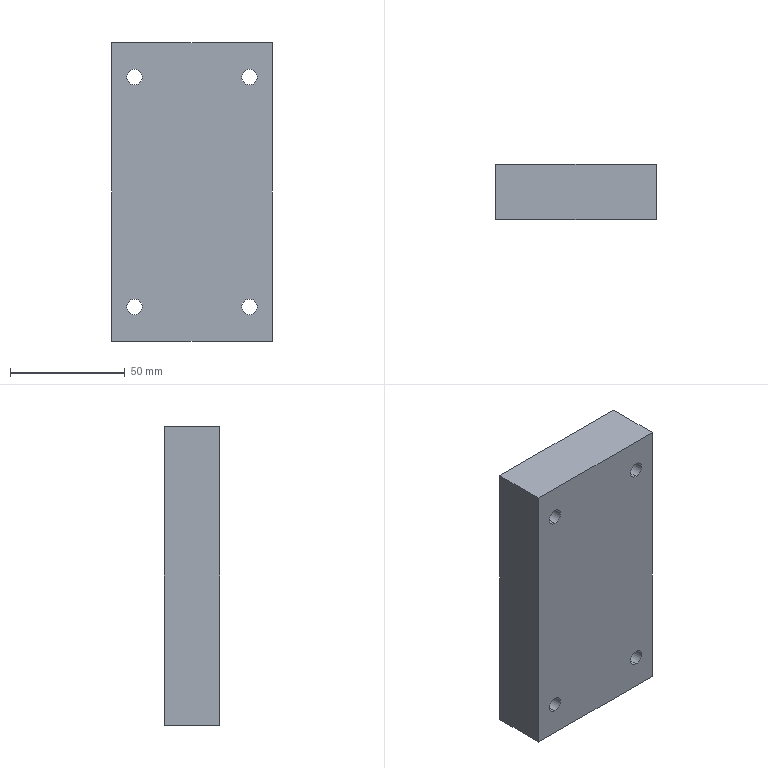Part | SolidWorks | features Extrusion 1, HoleWzd 1 | 1 solid | 14 faces | box 70 x 24 x 130 mm | volume 214914 mm3 | cylinder 8 | plane 6 | commonest cylinder face diameters 6.8 x8
STEP:
#1=CARTESIAN_POINT('',(-25.,0.,46.6));
#2=VERTEX_POINT('',#1);
#3=CARTESIAN_POINT('',(-25.,0.,53.4));
#4=VERTEX_POINT('',#3);
#5=CARTESIAN_POINT('',(-25.,0.,50.));
#6=DIRECTION('',(0.,1.,0.));
#7=DIRECTION('',(0.,0.,1.));
#8=AXIS2_PLACEMENT_3D('',#5,#6,#7);
#9=CIRCLE('',#8,3.4);
#10=EDGE_CURVE('',#2,#4,#9,.T.);
#11=ORIENTED_EDGE('',*,*,#10,.F.);
#12=CARTESIAN_POINT('',(-25.,24.,46.6));
#13=VERTEX_POINT('',#12);
#14=CARTESIAN_POINT('',(-25.,24.,46.6));
#15=DIRECTION('',(0.,1.,0.));
#16=VECTOR('',#15,1000.);
#17=LINE('',#14,#16);
#18=EDGE_CURVE('',#2,#13,#17,.T.);
#19=ORIENTED_EDGE('',*,*,#18,.T.);
#20=CARTESIAN_POINT('',(-25.,24.,53.4));
#21=VERTEX_POINT('',#20);
#22=CARTESIAN_POINT('',(-25.,24.,50.));
#23=DIRECTION('',(0.,1.,0.));
#24=DIRECTION('',(0.,0.,1.));
#25=AXIS2_PLACEMENT_3D('',#22,#23,#24);
#26=CIRCLE('',#25,3.4);
#27=EDGE_CURVE('',#13,#21,#26,.T.);
#28=ORIENTED_EDGE('',*,*,#27,.T.);
#29=CARTESIAN_POINT('',(-25.,24.,53.4));
#30=DIRECTION('',(0.,1.,0.));
#31=VECTOR('',#30,1000.);
#32=LINE('',#29,#31);
#33=EDGE_CURVE('',#4,#21,#32,.T.);
#34=ORIENTED_EDGE('',*,*,#33,.F.);
#35=EDGE_LOOP('',(#11,#19,#28,#34));
#36=FACE_OUTER_BOUND('',#35,.T.);
#37=CARTESIAN_POINT('',(-25.,24.,50.));
#38=DIRECTION('',(0.,1.,0.));
#39=DIRECTION('',(0.,0.,1.));
#40=AXIS2_PLACEMENT_3D('',#37,#38,#39);
#41=CYLINDRICAL_SURFACE('',#40,3.4);
#42=ADVANCED_FACE('',(#36),#41,.F.);
#43=CARTESIAN_POINT('',(-25.,0.,-53.4));
#44=VERTEX_POINT('',#43);
#45=CARTESIAN_POINT('',(-25.,0.,-46.6));
#46=VERTEX_POINT('',#45);
#47=CARTESIAN_POINT('',(-25.,0.,-50.));
#48=DIRECTION('',(0.,1.,0.));
#49=DIRECTION('',(0.,0.,1.));
#50=AXIS2_PLACEMENT_3D('',#47,#48,#49);
#51=CIRCLE('',#50,3.4);
#52=EDGE_CURVE('',#44,#46,#51,.T.);
#53=ORIENTED_EDGE('',*,*,#52,.F.);
#54=CARTESIAN_POINT('',(-25.,24.,-53.4));
#55=VERTEX_POINT('',#54);
#56=CARTESIAN_POINT('',(-25.,24.,-53.4));
#57=DIRECTION('',(0.,1.,0.));
#58=VECTOR('',#57,1000.);
#59=LINE('',#56,#58);
#60=EDGE_CURVE('',#44,#55,#59,.T.);
#61=ORIENTED_EDGE('',*,*,#60,.T.);
#62=CARTESIAN_POINT('',(-25.,24.,-46.6));
#63=VERTEX_POINT('',#62);
#64=CARTESIAN_POINT('',(-25.,24.,-50.));
#65=DIRECTION('',(0.,1.,0.));
#66=DIRECTION('',(0.,0.,1.));
#67=AXIS2_PLACEMENT_3D('',#64,#65,#66);
#68=CIRCLE('',#67,3.4);
#69=EDGE_CURVE('',#55,#63,#68,.T.);
#70=ORIENTED_EDGE('',*,*,#69,.T.);
#71=CARTESIAN_POINT('',(-25.,24.,-46.6));
#72=DIRECTION('',(0.,1.,0.));
#73=VECTOR('',#72,1000.);
#74=LINE('',#71,#73);
#75=EDGE_CURVE('',#46,#63,#74,.T.);
#76=ORIENTED_EDGE('',*,*,#75,.F.);
#77=EDGE_LOOP('',(#53,#61,#70,#76));
#78=FACE_OUTER_BOUND('',#77,.T.);
#79=CARTESIAN_POINT('',(-25.,24.,-50.));
#80=DIRECTION('',(0.,1.,0.));
#81=DIRECTION('',(0.,0.,1.));
#82=AXIS2_PLACEMENT_3D('',#79,#80,#81);
#83=CYLINDRICAL_SURFACE('',#82,3.4);
#84=ADVANCED_FACE('',(#78),#83,.F.);
#85=CARTESIAN_POINT('',(25.,0.,-53.4));
#86=VERTEX_POINT('',#85);
#87=CARTESIAN_POINT('',(25.,0.,-46.6));
#88=VERTEX_POINT('',#87);
#89=CARTESIAN_POINT('',(25.,0.,-50.));
#90=DIRECTION('',(0.,1.,0.));
#91=DIRECTION('',(0.,0.,1.));
#92=AXIS2_PLACEMENT_3D('',#89,#90,#91);
#93=CIRCLE('',#92,3.4);
#94=EDGE_CURVE('',#86,#88,#93,.T.);
#95=ORIENTED_EDGE('',*,*,#94,.F.);
#96=CARTESIAN_POINT('',(25.,24.,-53.4));
#97=VERTEX_POINT('',#96);
#98=CARTESIAN_POINT('',(25.,24.,-53.4));
#99=DIRECTION('',(0.,1.,0.));
#100=VECTOR('',#99,1000.);
#101=LINE('',#98,#100);
#102=EDGE_CURVE('',#86,#97,#101,.T.);
#103=ORIENTED_EDGE('',*,*,#102,.T.);
#104=CARTESIAN_POINT('',(25.,24.,-46.6));
#105=VERTEX_POINT('',#104);
#106=CARTESIAN_POINT('',(25.,24.,-50.));
#107=DIRECTION('',(0.,1.,0.));
#108=DIRECTION('',(0.,0.,1.));
#109=AXIS2_PLACEMENT_3D('',#106,#107,#108);
#110=CIRCLE('',#109,3.4);
#111=EDGE_CURVE('',#97,#105,#110,.T.);
#112=ORIENTED_EDGE('',*,*,#111,.T.);
#113=CARTESIAN_POINT('',(25.,24.,-46.6));
#114=DIRECTION('',(0.,1.,0.));
#115=VECTOR('',#114,1000.);
#116=LINE('',#113,#115);
#117=EDGE_CURVE('',#88,#105,#116,.T.);
#118=ORIENTED_EDGE('',*,*,#117,.F.);
#119=EDGE_LOOP('',(#95,#103,#112,#118));
#120=FACE_OUTER_BOUND('',#119,.T.);
#121=CARTESIAN_POINT('',(25.,24.,-50.));
#122=DIRECTION('',(0.,1.,0.));
#123=DIRECTION('',(0.,0.,1.));
#124=AXIS2_PLACEMENT_3D('',#121,#122,#123);
#125=CYLINDRICAL_SURFACE('',#124,3.4);
#126=ADVANCED_FACE('',(#120),#125,.F.);
#127=CARTESIAN_POINT('',(25.,0.,46.6));
#128=VERTEX_POINT('',#127);
#129=CARTESIAN_POINT('',(25.,0.,53.4));
#130=VERTEX_POINT('',#129);
#131=CARTESIAN_POINT('',(25.,0.,50.));
#132=DIRECTION('',(0.,1.,0.));
#133=DIRECTION('',(0.,0.,1.));
#134=AXIS2_PLACEMENT_3D('',#131,#132,#133);
#135=CIRCLE('',#134,3.4);
#136=EDGE_CURVE('',#128,#130,#135,.T.);
#137=ORIENTED_EDGE('',*,*,#136,.F.);
#138=CARTESIAN_POINT('',(25.,24.,46.6));
#139=VERTEX_POINT('',#138);
#140=CARTESIAN_POINT('',(25.,24.,46.6));
#141=DIRECTION('',(0.,1.,0.));
#142=VECTOR('',#141,1000.);
#143=LINE('',#140,#142);
#144=EDGE_CURVE('',#128,#139,#143,.T.);
#145=ORIENTED_EDGE('',*,*,#144,.T.);
#146=CARTESIAN_POINT('',(25.,24.,53.4));
#147=VERTEX_POINT('',#146);
#148=CARTESIAN_POINT('',(25.,24.,50.));
#149=DIRECTION('',(0.,1.,0.));
#150=DIRECTION('',(0.,0.,1.));
#151=AXIS2_PLACEMENT_3D('',#148,#149,#150);
#152=CIRCLE('',#151,3.4);
#153=EDGE_CURVE('',#139,#147,#152,.T.);
#154=ORIENTED_EDGE('',*,*,#153,.T.);
#155=CARTESIAN_POINT('',(25.,24.,53.4));
#156=DIRECTION('',(0.,1.,0.));
#157=VECTOR('',#156,1000.);
#158=LINE('',#155,#157);
#159=EDGE_CURVE('',#130,#147,#158,.T.);
#160=ORIENTED_EDGE('',*,*,#159,.F.);
#161=EDGE_LOOP('',(#137,#145,#154,#160));
#162=FACE_OUTER_BOUND('',#161,.T.);
#163=CARTESIAN_POINT('',(25.,24.,50.));
#164=DIRECTION('',(0.,1.,0.));
#165=DIRECTION('',(0.,0.,1.));
#166=AXIS2_PLACEMENT_3D('',#163,#164,#165);
#167=CYLINDRICAL_SURFACE('',#166,3.4);
#168=ADVANCED_FACE('',(#162),#167,.F.);
#169=CARTESIAN_POINT('',(35.,0.,65.));
#170=VERTEX_POINT('',#169);
#171=CARTESIAN_POINT('',(35.,0.,-65.));
#172=VERTEX_POINT('',#171);
#173=CARTESIAN_POINT('',(35.,0.,65.));
#174=DIRECTION('',(0.,0.,-1.));
#175=VECTOR('',#174,1000.);
#176=LINE('',#173,#175);
#177=EDGE_CURVE('',#170,#172,#176,.T.);
#178=ORIENTED_EDGE('',*,*,#177,.T.);
#179=CARTESIAN_POINT('',(35.,24.,-65.));
#180=VERTEX_POINT('',#179);
#181=CARTESIAN_POINT('',(35.,24.,-65.));
#182=DIRECTION('',(0.,-1.,0.));
#183=VECTOR('',#182,1000.);
#184=LINE('',#181,#183);
#185=EDGE_CURVE('',#180,#172,#184,.T.);
#186=ORIENTED_EDGE('',*,*,#185,.F.);
#187=CARTESIAN_POINT('',(35.,24.,65.));
#188=VERTEX_POINT('',#187);
#189=CARTESIAN_POINT('',(35.,24.,65.));
#190=DIRECTION('',(0.,0.,-1.));
#191=VECTOR('',#190,1000.);
#192=LINE('',#189,#191);
#193=EDGE_CURVE('',#188,#180,#192,.T.);
#194=ORIENTED_EDGE('',*,*,#193,.F.);
#195=CARTESIAN_POINT('',(35.,24.,65.));
#196=DIRECTION('',(0.,-1.,0.));
#197=VECTOR('',#196,1000.);
#198=LINE('',#195,#197);
#199=EDGE_CURVE('',#188,#170,#198,.T.);
#200=ORIENTED_EDGE('',*,*,#199,.T.);
#201=EDGE_LOOP('',(#178,#186,#194,#200));
#202=FACE_OUTER_BOUND('',#201,.T.);
#203=CARTESIAN_POINT('',(35.,24.,65.));
#204=DIRECTION('',(-1.,0.,0.));
#205=DIRECTION('',(0.,0.,1.));
#206=AXIS2_PLACEMENT_3D('',#203,#204,#205);
#207=PLANE('',#206);
#208=ADVANCED_FACE('',(#202),#207,.F.);
#209=CARTESIAN_POINT('',(-35.,0.,-65.));
#210=VERTEX_POINT('',#209);
#211=CARTESIAN_POINT('',(-35.,0.,-65.));
#212=DIRECTION('',(-1.,0.,0.));
#213=VECTOR('',#212,1000.);
#214=LINE('',#211,#213);
#215=EDGE_CURVE('',#172,#210,#214,.T.);
#216=ORIENTED_EDGE('',*,*,#215,.T.);
#217=CARTESIAN_POINT('',(-35.,24.,-65.));
#218=VERTEX_POINT('',#217);
#219=CARTESIAN_POINT('',(-35.,24.,-65.));
#220=DIRECTION('',(0.,-1.,0.));
#221=VECTOR('',#220,1000.);
#222=LINE('',#219,#221);
#223=EDGE_CURVE('',#218,#210,#222,.T.);
#224=ORIENTED_EDGE('',*,*,#223,.F.);
#225=CARTESIAN_POINT('',(-35.,24.,-65.));
#226=DIRECTION('',(-1.,0.,0.));
#227=VECTOR('',#226,1000.);
#228=LINE('',#225,#227);
#229=EDGE_CURVE('',#180,#218,#228,.T.);
#230=ORIENTED_EDGE('',*,*,#229,.F.);
#231=ORIENTED_EDGE('',*,*,#185,.T.);
#232=EDGE_LOOP('',(#216,#224,#230,#231));
#233=FACE_OUTER_BOUND('',#232,.T.);
#234=CARTESIAN_POINT('',(-35.,24.,-65.));
#235=DIRECTION('',(0.,0.,1.));
#236=DIRECTION('',(1.,0.,0.));
#237=AXIS2_PLACEMENT_3D('',#234,#235,#236);
#238=PLANE('',#237);
#239=ADVANCED_FACE('',(#233),#238,.F.);
#240=CARTESIAN_POINT('',(-35.,0.,65.));
#241=VERTEX_POINT('',#240);
#242=CARTESIAN_POINT('',(-35.,0.,65.));
#243=DIRECTION('',(0.,0.,1.));
#244=VECTOR('',#243,1000.);
#245=LINE('',#242,#244);
#246=EDGE_CURVE('',#210,#241,#245,.T.);
#247=ORIENTED_EDGE('',*,*,#246,.T.);
#248=CARTESIAN_POINT('',(-35.,24.,65.));
#249=VERTEX_POINT('',#248);
#250=CARTESIAN_POINT('',(-35.,24.,65.));
#251=DIRECTION('',(0.,-1.,0.));
#252=VECTOR('',#251,1000.);
#253=LINE('',#250,#252);
#254=EDGE_CURVE('',#249,#241,#253,.T.);
#255=ORIENTED_EDGE('',*,*,#254,.F.);
#256=CARTESIAN_POINT('',(-35.,24.,65.));
#257=DIRECTION('',(0.,0.,1.));
#258=VECTOR('',#257,1000.);
#259=LINE('',#256,#258);
#260=EDGE_CURVE('',#218,#249,#259,.T.);
#261=ORIENTED_EDGE('',*,*,#260,.F.);
#262=ORIENTED_EDGE('',*,*,#223,.T.);
#263=EDGE_LOOP('',(#247,#255,#261,#262));
#264=FACE_OUTER_BOUND('',#263,.T.);
#265=CARTESIAN_POINT('',(-35.,24.,65.));
#266=DIRECTION('',(1.,0.,0.));
#267=DIRECTION('',(0.,0.,-1.));
#268=AXIS2_PLACEMENT_3D('',#265,#266,#267);
#269=PLANE('',#268);
#270=ADVANCED_FACE('',(#264),#269,.F.);
#271=CARTESIAN_POINT('',(-35.,0.,65.));
#272=DIRECTION('',(1.,0.,0.));
#273=VECTOR('',#272,1000.);
#274=LINE('',#271,#273);
#275=EDGE_CURVE('',#241,#170,#274,.T.);
#276=ORIENTED_EDGE('',*,*,#275,.T.);
#277=ORIENTED_EDGE('',*,*,#199,.F.);
#278=CARTESIAN_POINT('',(-35.,24.,65.));
#279=DIRECTION('',(1.,0.,0.));
#280=VECTOR('',#279,1000.);
#281=LINE('',#278,#280);
#282=EDGE_CURVE('',#249,#188,#281,.T.);
#283=ORIENTED_EDGE('',*,*,#282,.F.);
#284=ORIENTED_EDGE('',*,*,#254,.T.);
#285=EDGE_LOOP('',(#276,#277,#283,#284));
#286=FACE_OUTER_BOUND('',#285,.T.);
#287=CARTESIAN_POINT('',(-35.,24.,65.));
#288=DIRECTION('',(0.,0.,-1.));
#289=DIRECTION('',(-1.,0.,0.));
#290=AXIS2_PLACEMENT_3D('',#287,#288,#289);
#291=PLANE('',#290);
#292=ADVANCED_FACE('',(#286),#291,.F.);
#293=CARTESIAN_POINT('',(-25.,24.,50.));
#294=DIRECTION('',(0.,1.,0.));
#295=DIRECTION('',(0.,0.,1.));
#296=AXIS2_PLACEMENT_3D('',#293,#294,#295);
#297=CIRCLE('',#296,3.4);
#298=EDGE_CURVE('',#21,#13,#297,.T.);
#299=ORIENTED_EDGE('',*,*,#298,.F.);
#300=ORIENTED_EDGE('',*,*,#27,.F.);
#301=EDGE_LOOP('',(#299,#300));
#302=FACE_BOUND('',#301,.T.);
#303=CARTESIAN_POINT('',(-25.,24.,-50.));
#304=DIRECTION('',(0.,1.,0.));
#305=DIRECTION('',(0.,0.,1.));
#306=AXIS2_PLACEMENT_3D('',#303,#304,#305);
#307=CIRCLE('',#306,3.4);
#308=EDGE_CURVE('',#63,#55,#307,.T.);
#309=ORIENTED_EDGE('',*,*,#308,.F.);
#310=ORIENTED_EDGE('',*,*,#69,.F.);
#311=EDGE_LOOP('',(#309,#310));
#312=FACE_BOUND('',#311,.T.);
#313=CARTESIAN_POINT('',(25.,24.,-50.));
#314=DIRECTION('',(0.,1.,0.));
#315=DIRECTION('',(0.,0.,1.));
#316=AXIS2_PLACEMENT_3D('',#313,#314,#315);
#317=CIRCLE('',#316,3.4);
#318=EDGE_CURVE('',#105,#97,#317,.T.);
#319=ORIENTED_EDGE('',*,*,#318,.F.);
#320=ORIENTED_EDGE('',*,*,#111,.F.);
#321=EDGE_LOOP('',(#319,#320));
#322=FACE_BOUND('',#321,.T.);
#323=CARTESIAN_POINT('',(25.,24.,50.));
#324=DIRECTION('',(0.,1.,0.));
#325=DIRECTION('',(0.,0.,1.));
#326=AXIS2_PLACEMENT_3D('',#323,#324,#325);
#327=CIRCLE('',#326,3.4);
#328=EDGE_CURVE('',#147,#139,#327,.T.);
#329=ORIENTED_EDGE('',*,*,#328,.F.);
#330=ORIENTED_EDGE('',*,*,#153,.F.);
#331=EDGE_LOOP('',(#329,#330));
#332=FACE_BOUND('',#331,.T.);
#333=ORIENTED_EDGE('',*,*,#193,.T.);
#334=ORIENTED_EDGE('',*,*,#229,.T.);
#335=ORIENTED_EDGE('',*,*,#260,.T.);
#336=ORIENTED_EDGE('',*,*,#282,.T.);
#337=EDGE_LOOP('',(#333,#334,#335,#336));
#338=FACE_OUTER_BOUND('',#337,.T.);
#339=CARTESIAN_POINT('',(0.,24.,0.));
#340=DIRECTION('',(0.,-1.,0.));
#341=DIRECTION('',(0.,0.,-1.));
#342=AXIS2_PLACEMENT_3D('',#339,#340,#341);
#343=PLANE('',#342);
#344=ADVANCED_FACE('',(#302,#312,#322,#332,#338),#343,.F.);
#345=CARTESIAN_POINT('',(-25.,0.,50.));
#346=DIRECTION('',(0.,1.,0.));
#347=DIRECTION('',(0.,0.,1.));
#348=AXIS2_PLACEMENT_3D('',#345,#346,#347);
#349=CIRCLE('',#348,3.4);
#350=EDGE_CURVE('',#4,#2,#349,.T.);
#351=ORIENTED_EDGE('',*,*,#350,.T.);
#352=ORIENTED_EDGE('',*,*,#10,.T.);
#353=EDGE_LOOP('',(#351,#352));
#354=FACE_BOUND('',#353,.T.);
#355=CARTESIAN_POINT('',(-25.,0.,-50.));
#356=DIRECTION('',(0.,1.,0.));
#357=DIRECTION('',(0.,0.,1.));
#358=AXIS2_PLACEMENT_3D('',#355,#356,#357);
#359=CIRCLE('',#358,3.4);
#360=EDGE_CURVE('',#46,#44,#359,.T.);
#361=ORIENTED_EDGE('',*,*,#360,.T.);
#362=ORIENTED_EDGE('',*,*,#52,.T.);
#363=EDGE_LOOP('',(#361,#362));
#364=FACE_BOUND('',#363,.T.);
#365=CARTESIAN_POINT('',(25.,0.,-50.));
#366=DIRECTION('',(0.,1.,0.));
#367=DIRECTION('',(0.,0.,1.));
#368=AXIS2_PLACEMENT_3D('',#365,#366,#367);
#369=CIRCLE('',#368,3.4);
#370=EDGE_CURVE('',#88,#86,#369,.T.);
#371=ORIENTED_EDGE('',*,*,#370,.T.);
#372=ORIENTED_EDGE('',*,*,#94,.T.);
#373=EDGE_LOOP('',(#371,#372));
#374=FACE_BOUND('',#373,.T.);
#375=CARTESIAN_POINT('',(25.,0.,50.));
#376=DIRECTION('',(0.,1.,0.));
#377=DIRECTION('',(0.,0.,1.));
#378=AXIS2_PLACEMENT_3D('',#375,#376,#377);
#379=CIRCLE('',#378,3.4);
#380=EDGE_CURVE('',#130,#128,#379,.T.);
#381=ORIENTED_EDGE('',*,*,#380,.T.);
#382=ORIENTED_EDGE('',*,*,#136,.T.);
#383=EDGE_LOOP('',(#381,#382));
#384=FACE_BOUND('',#383,.T.);
#385=ORIENTED_EDGE('',*,*,#177,.F.);
#386=ORIENTED_EDGE('',*,*,#275,.F.);
#387=ORIENTED_EDGE('',*,*,#246,.F.);
#388=ORIENTED_EDGE('',*,*,#215,.F.);
#389=EDGE_LOOP('',(#385,#386,#387,#388));
#390=FACE_OUTER_BOUND('',#389,.T.);
#391=CARTESIAN_POINT('',(0.,0.,0.));
#392=DIRECTION('',(0.,-1.,0.));
#393=DIRECTION('',(0.,0.,-1.));
#394=AXIS2_PLACEMENT_3D('',#391,#392,#393);
#395=PLANE('',#394);
#396=ADVANCED_FACE('',(#354,#364,#374,#384,#390),#395,.T.);
#397=ORIENTED_EDGE('',*,*,#144,.F.);
#398=ORIENTED_EDGE('',*,*,#380,.F.);
#399=ORIENTED_EDGE('',*,*,#159,.T.);
#400=ORIENTED_EDGE('',*,*,#328,.T.);
#401=EDGE_LOOP('',(#397,#398,#399,#400));
#402=FACE_OUTER_BOUND('',#401,.T.);
#403=CARTESIAN_POINT('',(25.,24.,50.));
#404=DIRECTION('',(0.,1.,0.));
#405=DIRECTION('',(0.,0.,1.));
#406=AXIS2_PLACEMENT_3D('',#403,#404,#405);
#407=CYLINDRICAL_SURFACE('',#406,3.4);
#408=ADVANCED_FACE('',(#402),#407,.F.);
#409=ORIENTED_EDGE('',*,*,#102,.F.);
#410=ORIENTED_EDGE('',*,*,#370,.F.);
#411=ORIENTED_EDGE('',*,*,#117,.T.);
#412=ORIENTED_EDGE('',*,*,#318,.T.);
#413=EDGE_LOOP('',(#409,#410,#411,#412));
#414=FACE_OUTER_BOUND('',#413,.T.);
#415=CARTESIAN_POINT('',(25.,24.,-50.));
#416=DIRECTION('',(0.,1.,0.));
#417=DIRECTION('',(0.,0.,1.));
#418=AXIS2_PLACEMENT_3D('',#415,#416,#417);
#419=CYLINDRICAL_SURFACE('',#418,3.4);
#420=ADVANCED_FACE('',(#414),#419,.F.);
#421=ORIENTED_EDGE('',*,*,#60,.F.);
#422=ORIENTED_EDGE('',*,*,#360,.F.);
#423=ORIENTED_EDGE('',*,*,#75,.T.);
#424=ORIENTED_EDGE('',*,*,#308,.T.);
#425=EDGE_LOOP('',(#421,#422,#423,#424));
#426=FACE_OUTER_BOUND('',#425,.T.);
#427=CARTESIAN_POINT('',(-25.,24.,-50.));
#428=DIRECTION('',(0.,1.,0.));
#429=DIRECTION('',(0.,0.,1.));
#430=AXIS2_PLACEMENT_3D('',#427,#428,#429);
#431=CYLINDRICAL_SURFACE('',#430,3.4);
#432=ADVANCED_FACE('',(#426),#431,.F.);
#433=ORIENTED_EDGE('',*,*,#18,.F.);
#434=ORIENTED_EDGE('',*,*,#350,.F.);
#435=ORIENTED_EDGE('',*,*,#33,.T.);
#436=ORIENTED_EDGE('',*,*,#298,.T.);
#437=EDGE_LOOP('',(#433,#434,#435,#436));
#438=FACE_OUTER_BOUND('',#437,.T.);
#439=CARTESIAN_POINT('',(-25.,24.,50.));
#440=DIRECTION('',(0.,1.,0.));
#441=DIRECTION('',(0.,0.,1.));
#442=AXIS2_PLACEMENT_3D('',#439,#440,#441);
#443=CYLINDRICAL_SURFACE('',#442,3.4);
#444=ADVANCED_FACE('',(#438),#443,.F.);
#445=CLOSED_SHELL('',(#42,#84,#126,#168,#208,#239,#270,#292,#344,#396,#408,#420,#432,#444));
#446=MANIFOLD_SOLID_BREP('',#445);
#447=CARTESIAN_POINT('',(0.,0.,0.));
#448=DIRECTION('',(0.,0.,1.));
#449=DIRECTION('',(1.,0.,0.));
#450=AXIS2_PLACEMENT_3D('',#447,#448,#449);
#451=(LENGTH_UNIT()NAMED_UNIT(*)SI_UNIT(.MILLI.,.METRE.));
#452=UNCERTAINTY_MEASURE_WITH_UNIT(LENGTH_MEASURE(0.00001),#451,'','');
#453=(NAMED_UNIT(*)PLANE_ANGLE_UNIT()SI_UNIT($,.RADIAN.));
#454=(NAMED_UNIT(*)SI_UNIT($,.STERADIAN.)SOLID_ANGLE_UNIT());
#455=(GEOMETRIC_REPRESENTATION_CONTEXT(3)GLOBAL_UNCERTAINTY_ASSIGNED_CONTEXT((#452))GLOBAL_UNIT_ASSIGNED_CONTEXT((#451,#453,#454))REPRESENTATION_CONTEXT('',''));
#456=ADVANCED_BREP_SHAPE_REPRESENTATION('',(#446,#450),#455);